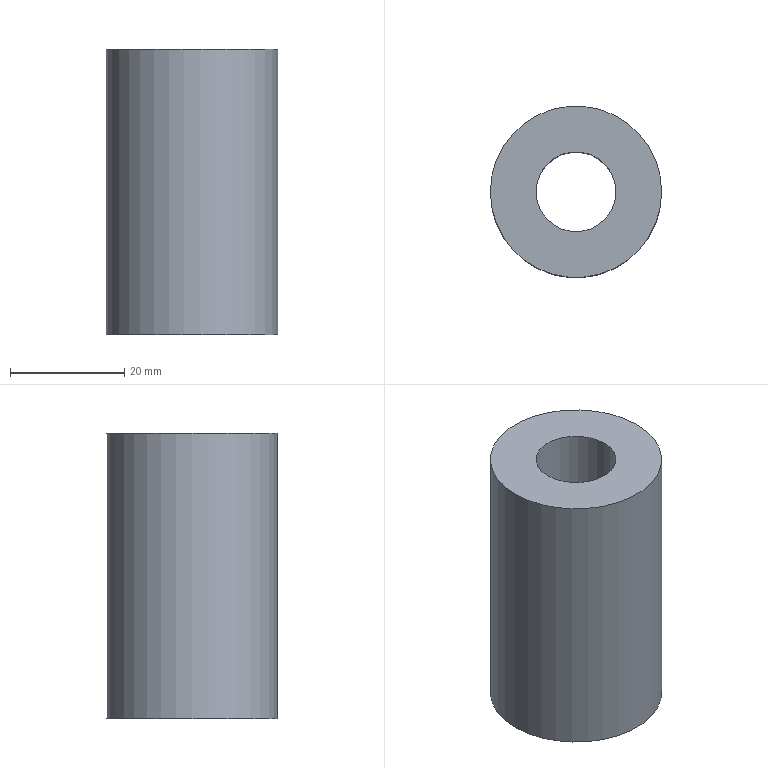Part | NX | features solid 2 | 1 solid | 4 faces | box 30 x 30 x 50 mm | volume 27646 mm3 | plane 2 | cylinder 2 | commonest cylinder face diameters 14 x1 30 x1
STEP:
#1=CARTESIAN_POINT('',(-545.,20.,-62.));
#2=VERTEX_POINT('',#1);
#3=CARTESIAN_POINT('',(-560.,20.,-62.));
#4=DIRECTION('',(0.,0.,1.));
#5=DIRECTION('',(1.,0.,0.));
#6=AXIS2_PLACEMENT_3D('',#3,#4,#5);
#7=CIRCLE('',#6,15.);
#8=EDGE_CURVE('',#2,#2,#7,.T.);
#9=ORIENTED_EDGE('',*,*,#8,.F.);
#10=EDGE_LOOP('',(#9));
#11=FACE_BOUND('',#10,.T.);
#12=CARTESIAN_POINT('',(-553.,20.,-62.));
#13=VERTEX_POINT('',#12);
#14=CARTESIAN_POINT('',(-560.,20.,-62.));
#15=DIRECTION('',(0.,0.,1.));
#16=DIRECTION('',(1.,0.,0.));
#17=AXIS2_PLACEMENT_3D('',#14,#15,#16);
#18=CIRCLE('',#17,7.);
#19=EDGE_CURVE('',#13,#13,#18,.F.);
#20=ORIENTED_EDGE('',*,*,#19,.F.);
#21=EDGE_LOOP('',(#20));
#22=FACE_BOUND('',#21,.T.);
#23=CARTESIAN_POINT('',(-560.,20.,-62.));
#24=DIRECTION('',(0.,0.,1.));
#25=DIRECTION('',(1.,0.,0.));
#26=AXIS2_PLACEMENT_3D('',#23,#24,#25);
#27=PLANE('',#26);
#28=ADVANCED_FACE('',(#11,#22),#27,.F.);
#29=CARTESIAN_POINT('',(-545.,20.,-12.));
#30=VERTEX_POINT('',#29);
#31=CARTESIAN_POINT('',(-560.,20.,-12.));
#32=DIRECTION('',(0.,0.,1.));
#33=DIRECTION('',(1.,0.,0.));
#34=AXIS2_PLACEMENT_3D('',#31,#32,#33);
#35=CIRCLE('',#34,15.);
#36=EDGE_CURVE('',#30,#30,#35,.T.);
#37=ORIENTED_EDGE('',*,*,#36,.T.);
#38=EDGE_LOOP('',(#37));
#39=FACE_BOUND('',#38,.T.);
#40=CARTESIAN_POINT('',(-553.,20.,-12.));
#41=VERTEX_POINT('',#40);
#42=CARTESIAN_POINT('',(-560.,20.,-12.));
#43=DIRECTION('',(0.,0.,1.));
#44=DIRECTION('',(1.,0.,0.));
#45=AXIS2_PLACEMENT_3D('',#42,#43,#44);
#46=CIRCLE('',#45,7.);
#47=EDGE_CURVE('',#41,#41,#46,.T.);
#48=ORIENTED_EDGE('',*,*,#47,.F.);
#49=EDGE_LOOP('',(#48));
#50=FACE_BOUND('',#49,.T.);
#51=CARTESIAN_POINT('',(-560.,20.,-12.));
#52=DIRECTION('',(0.,0.,1.));
#53=DIRECTION('',(1.,0.,0.));
#54=AXIS2_PLACEMENT_3D('',#51,#52,#53);
#55=PLANE('',#54);
#56=ADVANCED_FACE('',(#39,#50),#55,.T.);
#57=ORIENTED_EDGE('',*,*,#8,.T.);
#58=EDGE_LOOP('',(#57));
#59=FACE_BOUND('',#58,.T.);
#60=ORIENTED_EDGE('',*,*,#36,.F.);
#61=EDGE_LOOP('',(#60));
#62=FACE_BOUND('',#61,.T.);
#63=CARTESIAN_POINT('',(-560.,20.,-62.));
#64=DIRECTION('',(0.,0.,1.));
#65=DIRECTION('',(1.,0.,0.));
#66=AXIS2_PLACEMENT_3D('',#63,#64,#65);
#67=CYLINDRICAL_SURFACE('',#66,15.);
#68=ADVANCED_FACE('',(#59,#62),#67,.T.);
#69=ORIENTED_EDGE('',*,*,#47,.T.);
#70=EDGE_LOOP('',(#69));
#71=FACE_BOUND('',#70,.T.);
#72=ORIENTED_EDGE('',*,*,#19,.T.);
#73=EDGE_LOOP('',(#72));
#74=FACE_BOUND('',#73,.T.);
#75=CARTESIAN_POINT('',(-560.,20.,-12.));
#76=DIRECTION('',(0.,0.,-1.));
#77=DIRECTION('',(-1.,0.,0.));
#78=AXIS2_PLACEMENT_3D('',#75,#76,#77);
#79=CYLINDRICAL_SURFACE('',#78,7.);
#80=ADVANCED_FACE('',(#71,#74),#79,.F.);
#81=CLOSED_SHELL('',(#28,#56,#68,#80));
#82=MANIFOLD_SOLID_BREP('',#81);
#83=(LENGTH_UNIT()NAMED_UNIT(*)SI_UNIT(.MILLI.,.METRE.));
#84=UNCERTAINTY_MEASURE_WITH_UNIT(LENGTH_MEASURE(0.00001),#83,'','');
#85=(NAMED_UNIT(*)PLANE_ANGLE_UNIT()SI_UNIT($,.RADIAN.));
#86=(NAMED_UNIT(*)SI_UNIT($,.STERADIAN.)SOLID_ANGLE_UNIT());
#87=(GEOMETRIC_REPRESENTATION_CONTEXT(3)GLOBAL_UNCERTAINTY_ASSIGNED_CONTEXT((#84))GLOBAL_UNIT_ASSIGNED_CONTEXT((#83,#85,#86))REPRESENTATION_CONTEXT('',''));
#88=ADVANCED_BREP_SHAPE_REPRESENTATION('',(#82),#87);